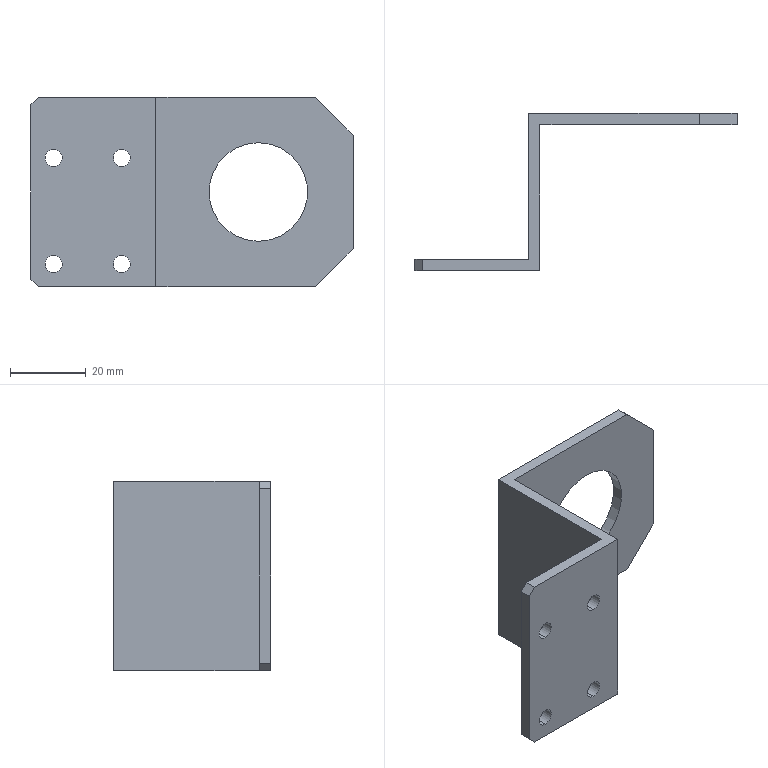Part | STEP file | rotary joint support 3.SLDDRW | 1 solid | 24 faces | box 85 x 41.5 x 50 mm | volume 16429 mm3 | plane 14 | cylinder 10 | commonest cylinder face diameters 4.5 x8 26 x2